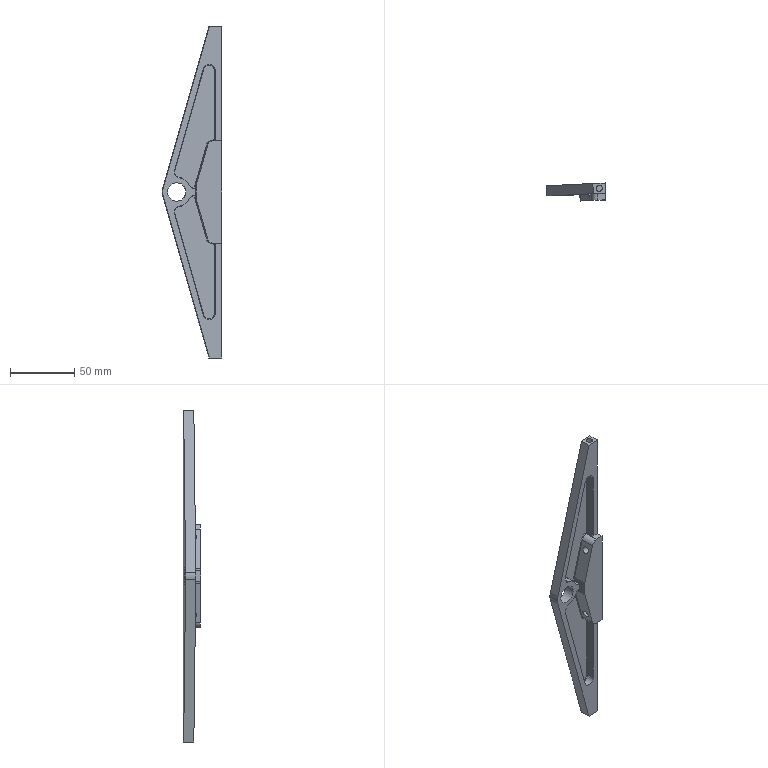Part | NX | features MG0317 steering brace 2 | 1 solid | 73 faces | box 46.441 x 13.827 x 258.318 mm | volume 40155 mm3 | cylinder 34 | plane 23 | torus 12 | sphere 4 | commonest cylinder face diameters 1.016 x16 9.525 x6 10 x4 22.225 x3 4.763 x2 5.41 x2